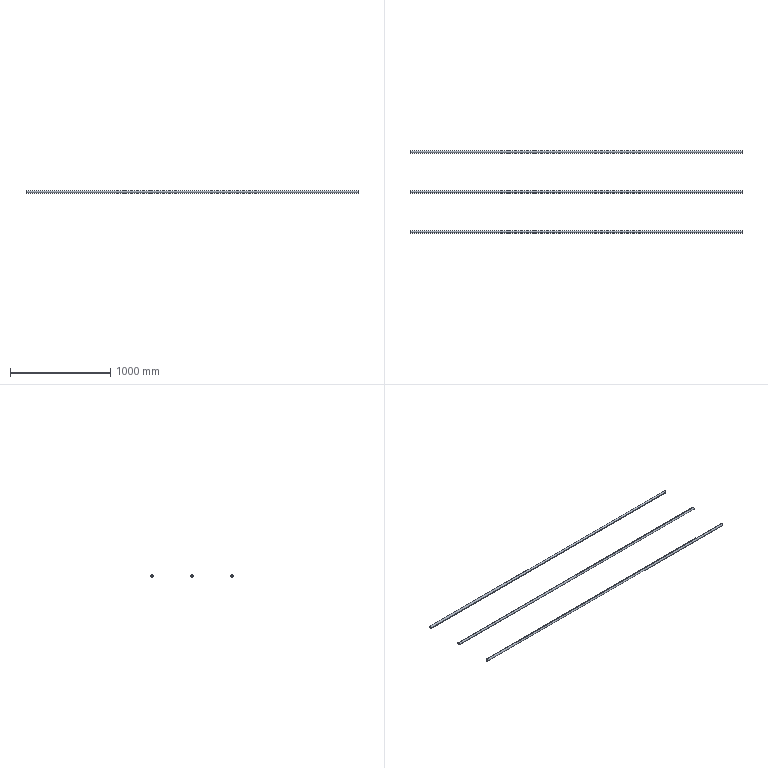Part | STEP file | E3-电柜护栏5栏杆_Default<As Machined> | 3 solids | 18 faces | box 3320 x 825 x 25 mm | volume 1102982 mm3 | cylinder 12 | plane 6 | commonest cylinder face diameters 22 x6 25 x6
STEP:
#1=CARTESIAN_POINT('',(0.,0.,0.));
#2=DIRECTION('',(0.,0.,1.));
#3=DIRECTION('',(1.,0.,0.));
#4=AXIS2_PLACEMENT_3D('',#1,#2,#3);
#5=CARTESIAN_POINT('',(-3320.,0.,12.5));
#6=VERTEX_POINT('',#5);
#7=CARTESIAN_POINT('',(-3320.,0.,-12.5));
#8=VERTEX_POINT('',#7);
#9=CARTESIAN_POINT('',(-3320.,0.,0.));
#10=DIRECTION('',(1.,0.,0.));
#11=DIRECTION('',(0.,-1.,0.));
#12=AXIS2_PLACEMENT_3D('',#9,#10,#11);
#13=CIRCLE('',#12,12.5);
#14=CARTESIAN_POINT('',(-3320.,0.,0.));
#15=DIRECTION('',(1.,0.,0.));
#16=DIRECTION('',(0.,0.,1.));
#17=AXIS2_PLACEMENT_3D('',#14,#15,#16);
#18=CYLINDRICAL_SURFACE('',#17,12.5);
#19=CARTESIAN_POINT('',(-4.712,0.));
#20=DIRECTION('',(1.,0.));
#21=VECTOR('',#20,1.);
#22=LINE('',#19,#21);
#23=(GEOMETRIC_REPRESENTATION_CONTEXT(2)PARAMETRIC_REPRESENTATION_CONTEXT()REPRESENTATION_CONTEXT('',''));
#24=DEFINITIONAL_REPRESENTATION('',(#22),#23);
#25=PCURVE('',#18,#24);
#26=CARTESIAN_POINT('',(-3320.,0.,0.));
#27=DIRECTION('',(-1.,0.,0.));
#28=DIRECTION('',(0.,-1.,0.));
#29=AXIS2_PLACEMENT_3D('',#26,#27,#28);
#30=PLANE('',#29);
#31=CARTESIAN_POINT('',(12.5,0.));
#32=CARTESIAN_POINT('',(12.5,-21.651));
#33=CARTESIAN_POINT('',(-6.25,-10.825));
#34=CARTESIAN_POINT('',(-25.,0.));
#35=CARTESIAN_POINT('',(-6.25,10.825));
#36=CARTESIAN_POINT('',(12.5,21.651));
#37=CARTESIAN_POINT('',(12.5,0.));
#38=(BOUNDED_CURVE()B_SPLINE_CURVE(2,(#31,#32,#33,#34,#35,#36,#37),.UNSPECIFIED.,.T.,.F.)B_SPLINE_CURVE_WITH_KNOTS((1,2,2,2,2,1),(-2.094,0.,2.094,4.189,6.283,8.378),.UNSPECIFIED.)CURVE()GEOMETRIC_REPRESENTATION_ITEM()RATIONAL_B_SPLINE_CURVE((1.,0.5,1.,0.5,1.,0.5,1.))REPRESENTATION_ITEM(''));
#39=(GEOMETRIC_REPRESENTATION_CONTEXT(2)PARAMETRIC_REPRESENTATION_CONTEXT()REPRESENTATION_CONTEXT('',''));
#40=DEFINITIONAL_REPRESENTATION('',(#38),#39);
#41=PCURVE('',#30,#40);
#42=SURFACE_CURVE('',#13,(#25,#41),.PCURVE_S1.);
#43=EDGE_CURVE('',#6,#8,#42,.T.);
#44=ORIENTED_EDGE('',*,*,#43,.T.);
#45=CARTESIAN_POINT('',(0.,0.,-12.5));
#46=VERTEX_POINT('',#45);
#47=CARTESIAN_POINT('',(-3320.,0.,-12.5));
#48=DIRECTION('',(1.,0.,0.));
#49=VECTOR('',#48,1.);
#50=LINE('',#47,#49);
#51=CARTESIAN_POINT('',(3.142,0.));
#52=DIRECTION('',(0.,1.));
#53=VECTOR('',#52,1.);
#54=LINE('',#51,#53);
#55=(GEOMETRIC_REPRESENTATION_CONTEXT(2)PARAMETRIC_REPRESENTATION_CONTEXT()REPRESENTATION_CONTEXT('',''));
#56=DEFINITIONAL_REPRESENTATION('',(#54),#55);
#57=PCURVE('',#18,#56);
#58=CARTESIAN_POINT('',(-3320.,0.,0.));
#59=DIRECTION('',(1.,0.,0.));
#60=DIRECTION('',(0.,0.,1.));
#61=AXIS2_PLACEMENT_3D('',#58,#59,#60);
#62=CYLINDRICAL_SURFACE('',#61,12.5);
#63=CARTESIAN_POINT('',(3.142,0.));
#64=DIRECTION('',(0.,1.));
#65=VECTOR('',#64,1.);
#66=LINE('',#63,#65);
#67=(GEOMETRIC_REPRESENTATION_CONTEXT(2)PARAMETRIC_REPRESENTATION_CONTEXT()REPRESENTATION_CONTEXT('',''));
#68=DEFINITIONAL_REPRESENTATION('',(#66),#67);
#69=PCURVE('',#62,#68);
#70=SURFACE_CURVE('',#50,(#57,#69),.PCURVE_S1.);
#71=EDGE_CURVE('',#8,#46,#70,.T.);
#72=ORIENTED_EDGE('',*,*,#71,.T.);
#73=CARTESIAN_POINT('',(0.,0.,12.5));
#74=VERTEX_POINT('',#73);
#75=CARTESIAN_POINT('',(0.,0.,0.));
#76=DIRECTION('',(1.,0.,0.));
#77=DIRECTION('',(0.,-1.,0.));
#78=AXIS2_PLACEMENT_3D('',#75,#76,#77);
#79=CIRCLE('',#78,12.5);
#80=CARTESIAN_POINT('',(-4.712,3320.));
#81=DIRECTION('',(1.,0.));
#82=VECTOR('',#81,1.);
#83=LINE('',#80,#82);
#84=(GEOMETRIC_REPRESENTATION_CONTEXT(2)PARAMETRIC_REPRESENTATION_CONTEXT()REPRESENTATION_CONTEXT('',''));
#85=DEFINITIONAL_REPRESENTATION('',(#83),#84);
#86=PCURVE('',#18,#85);
#87=CARTESIAN_POINT('',(0.,0.,0.));
#88=DIRECTION('',(-1.,0.,0.));
#89=DIRECTION('',(0.,-1.,0.));
#90=AXIS2_PLACEMENT_3D('',#87,#88,#89);
#91=PLANE('',#90);
#92=CARTESIAN_POINT('',(12.5,0.));
#93=CARTESIAN_POINT('',(12.5,-21.651));
#94=CARTESIAN_POINT('',(-6.25,-10.825));
#95=CARTESIAN_POINT('',(-25.,0.));
#96=CARTESIAN_POINT('',(-6.25,10.825));
#97=CARTESIAN_POINT('',(12.5,21.651));
#98=CARTESIAN_POINT('',(12.5,0.));
#99=(BOUNDED_CURVE()B_SPLINE_CURVE(2,(#92,#93,#94,#95,#96,#97,#98),.UNSPECIFIED.,.T.,.F.)B_SPLINE_CURVE_WITH_KNOTS((1,2,2,2,2,1),(-2.094,0.,2.094,4.189,6.283,8.378),.UNSPECIFIED.)CURVE()GEOMETRIC_REPRESENTATION_ITEM()RATIONAL_B_SPLINE_CURVE((1.,0.5,1.,0.5,1.,0.5,1.))REPRESENTATION_ITEM(''));
#100=(GEOMETRIC_REPRESENTATION_CONTEXT(2)PARAMETRIC_REPRESENTATION_CONTEXT()REPRESENTATION_CONTEXT('',''));
#101=DEFINITIONAL_REPRESENTATION('',(#99),#100);
#102=PCURVE('',#91,#101);
#103=SURFACE_CURVE('',#79,(#86,#102),.PCURVE_S1.);
#104=EDGE_CURVE('',#74,#46,#103,.T.);
#105=ORIENTED_EDGE('',*,*,#104,.F.);
#106=CARTESIAN_POINT('',(-3320.,0.,12.5));
#107=DIRECTION('',(1.,0.,0.));
#108=VECTOR('',#107,1.);
#109=LINE('',#106,#108);
#110=CARTESIAN_POINT('',(0.,0.));
#111=DIRECTION('',(0.,1.));
#112=VECTOR('',#111,1.);
#113=LINE('',#110,#112);
#114=(GEOMETRIC_REPRESENTATION_CONTEXT(2)PARAMETRIC_REPRESENTATION_CONTEXT()REPRESENTATION_CONTEXT('',''));
#115=DEFINITIONAL_REPRESENTATION('',(#113),#114);
#116=PCURVE('',#18,#115);
#117=CARTESIAN_POINT('',(6.283,0.));
#118=DIRECTION('',(0.,1.));
#119=VECTOR('',#118,1.);
#120=LINE('',#117,#119);
#121=(GEOMETRIC_REPRESENTATION_CONTEXT(2)PARAMETRIC_REPRESENTATION_CONTEXT()REPRESENTATION_CONTEXT('',''));
#122=DEFINITIONAL_REPRESENTATION('',(#120),#121);
#123=PCURVE('',#62,#122);
#124=SURFACE_CURVE('',#109,(#116,#123),.PCURVE_S1.);
#125=EDGE_CURVE('',#6,#74,#124,.T.);
#126=ORIENTED_EDGE('',*,*,#125,.F.);
#127=EDGE_LOOP('',(#44,#72,#105,#126));
#128=FACE_BOUND('',#127,.T.);
#129=ADVANCED_FACE('',(#128),#18,.T.);
#130=CARTESIAN_POINT('',(-3320.,0.,11.));
#131=VERTEX_POINT('',#130);
#132=CARTESIAN_POINT('',(0.,0.,11.));
#133=VERTEX_POINT('',#132);
#134=CARTESIAN_POINT('',(-3320.,0.,11.));
#135=DIRECTION('',(1.,0.,0.));
#136=VECTOR('',#135,1.);
#137=LINE('',#134,#136);
#138=CARTESIAN_POINT('',(-3320.,0.,0.));
#139=DIRECTION('',(1.,0.,0.));
#140=DIRECTION('',(0.,0.,1.));
#141=AXIS2_PLACEMENT_3D('',#138,#139,#140);
#142=CYLINDRICAL_SURFACE('',#141,11.);
#143=CARTESIAN_POINT('',(6.283,0.));
#144=DIRECTION('',(0.,1.));
#145=VECTOR('',#144,1.);
#146=LINE('',#143,#145);
#147=(GEOMETRIC_REPRESENTATION_CONTEXT(2)PARAMETRIC_REPRESENTATION_CONTEXT()REPRESENTATION_CONTEXT('',''));
#148=DEFINITIONAL_REPRESENTATION('',(#146),#147);
#149=PCURVE('',#142,#148);
#150=CARTESIAN_POINT('',(-3320.,0.,0.));
#151=DIRECTION('',(1.,0.,0.));
#152=DIRECTION('',(0.,0.,1.));
#153=AXIS2_PLACEMENT_3D('',#150,#151,#152);
#154=CYLINDRICAL_SURFACE('',#153,11.);
#155=CARTESIAN_POINT('',(0.,0.));
#156=DIRECTION('',(0.,1.));
#157=VECTOR('',#156,1.);
#158=LINE('',#155,#157);
#159=(GEOMETRIC_REPRESENTATION_CONTEXT(2)PARAMETRIC_REPRESENTATION_CONTEXT()REPRESENTATION_CONTEXT('',''));
#160=DEFINITIONAL_REPRESENTATION('',(#158),#159);
#161=PCURVE('',#154,#160);
#162=SURFACE_CURVE('',#137,(#149,#161),.PCURVE_S1.);
#163=EDGE_CURVE('',#131,#133,#162,.T.);
#164=ORIENTED_EDGE('',*,*,#163,.T.);
#165=CARTESIAN_POINT('',(0.,0.,-11.));
#166=VERTEX_POINT('',#165);
#167=CARTESIAN_POINT('',(0.,0.,0.));
#168=DIRECTION('',(1.,0.,0.));
#169=DIRECTION('',(0.,-1.,0.));
#170=AXIS2_PLACEMENT_3D('',#167,#168,#169);
#171=CIRCLE('',#170,11.);
#172=CARTESIAN_POINT('',(1.571,3320.));
#173=DIRECTION('',(1.,0.));
#174=VECTOR('',#173,1.);
#175=LINE('',#172,#174);
#176=(GEOMETRIC_REPRESENTATION_CONTEXT(2)PARAMETRIC_REPRESENTATION_CONTEXT()REPRESENTATION_CONTEXT('',''));
#177=DEFINITIONAL_REPRESENTATION('',(#175),#176);
#178=PCURVE('',#142,#177);
#179=CARTESIAN_POINT('',(11.,0.));
#180=CARTESIAN_POINT('',(11.,-19.053));
#181=CARTESIAN_POINT('',(-5.5,-9.526));
#182=CARTESIAN_POINT('',(-22.,0.));
#183=CARTESIAN_POINT('',(-5.5,9.526));
#184=CARTESIAN_POINT('',(11.,19.053));
#185=CARTESIAN_POINT('',(11.,0.));
#186=(BOUNDED_CURVE()B_SPLINE_CURVE(2,(#179,#180,#181,#182,#183,#184,#185),.UNSPECIFIED.,.T.,.F.)B_SPLINE_CURVE_WITH_KNOTS((1,2,2,2,2,1),(-2.094,0.,2.094,4.189,6.283,8.378),.UNSPECIFIED.)CURVE()GEOMETRIC_REPRESENTATION_ITEM()RATIONAL_B_SPLINE_CURVE((1.,0.5,1.,0.5,1.,0.5,1.))REPRESENTATION_ITEM(''));
#187=(GEOMETRIC_REPRESENTATION_CONTEXT(2)PARAMETRIC_REPRESENTATION_CONTEXT()REPRESENTATION_CONTEXT('',''));
#188=DEFINITIONAL_REPRESENTATION('',(#186),#187);
#189=PCURVE('',#91,#188);
#190=SURFACE_CURVE('',#171,(#178,#189),.PCURVE_S1.);
#191=EDGE_CURVE('',#166,#133,#190,.T.);
#192=ORIENTED_EDGE('',*,*,#191,.F.);
#193=CARTESIAN_POINT('',(-3320.,0.,-11.));
#194=VERTEX_POINT('',#193);
#195=CARTESIAN_POINT('',(-3320.,0.,-11.));
#196=DIRECTION('',(1.,0.,0.));
#197=VECTOR('',#196,1.);
#198=LINE('',#195,#197);
#199=CARTESIAN_POINT('',(3.142,0.));
#200=DIRECTION('',(0.,1.));
#201=VECTOR('',#200,1.);
#202=LINE('',#199,#201);
#203=(GEOMETRIC_REPRESENTATION_CONTEXT(2)PARAMETRIC_REPRESENTATION_CONTEXT()REPRESENTATION_CONTEXT('',''));
#204=DEFINITIONAL_REPRESENTATION('',(#202),#203);
#205=PCURVE('',#142,#204);
#206=CARTESIAN_POINT('',(3.142,0.));
#207=DIRECTION('',(0.,1.));
#208=VECTOR('',#207,1.);
#209=LINE('',#206,#208);
#210=(GEOMETRIC_REPRESENTATION_CONTEXT(2)PARAMETRIC_REPRESENTATION_CONTEXT()REPRESENTATION_CONTEXT('',''));
#211=DEFINITIONAL_REPRESENTATION('',(#209),#210);
#212=PCURVE('',#154,#211);
#213=SURFACE_CURVE('',#198,(#205,#212),.PCURVE_S1.);
#214=EDGE_CURVE('',#194,#166,#213,.T.);
#215=ORIENTED_EDGE('',*,*,#214,.F.);
#216=CARTESIAN_POINT('',(-3320.,0.,0.));
#217=DIRECTION('',(1.,0.,0.));
#218=DIRECTION('',(0.,-1.,0.));
#219=AXIS2_PLACEMENT_3D('',#216,#217,#218);
#220=CIRCLE('',#219,11.);
#221=CARTESIAN_POINT('',(1.571,0.));
#222=DIRECTION('',(1.,0.));
#223=VECTOR('',#222,1.);
#224=LINE('',#221,#223);
#225=(GEOMETRIC_REPRESENTATION_CONTEXT(2)PARAMETRIC_REPRESENTATION_CONTEXT()REPRESENTATION_CONTEXT('',''));
#226=DEFINITIONAL_REPRESENTATION('',(#224),#225);
#227=PCURVE('',#142,#226);
#228=CARTESIAN_POINT('',(11.,0.));
#229=CARTESIAN_POINT('',(11.,-19.053));
#230=CARTESIAN_POINT('',(-5.5,-9.526));
#231=CARTESIAN_POINT('',(-22.,0.));
#232=CARTESIAN_POINT('',(-5.5,9.526));
#233=CARTESIAN_POINT('',(11.,19.053));
#234=CARTESIAN_POINT('',(11.,0.));
#235=(BOUNDED_CURVE()B_SPLINE_CURVE(2,(#228,#229,#230,#231,#232,#233,#234),.UNSPECIFIED.,.T.,.F.)B_SPLINE_CURVE_WITH_KNOTS((1,2,2,2,2,1),(-2.094,0.,2.094,4.189,6.283,8.378),.UNSPECIFIED.)CURVE()GEOMETRIC_REPRESENTATION_ITEM()RATIONAL_B_SPLINE_CURVE((1.,0.5,1.,0.5,1.,0.5,1.))REPRESENTATION_ITEM(''));
#236=(GEOMETRIC_REPRESENTATION_CONTEXT(2)PARAMETRIC_REPRESENTATION_CONTEXT()REPRESENTATION_CONTEXT('',''));
#237=DEFINITIONAL_REPRESENTATION('',(#235),#236);
#238=PCURVE('',#30,#237);
#239=SURFACE_CURVE('',#220,(#227,#238),.PCURVE_S1.);
#240=EDGE_CURVE('',#194,#131,#239,.T.);
#241=ORIENTED_EDGE('',*,*,#240,.T.);
#242=EDGE_LOOP('',(#164,#192,#215,#241));
#243=FACE_BOUND('',#242,.F.);
#244=ADVANCED_FACE('',(#243),#142,.F.);
#245=CARTESIAN_POINT('',(0.,0.,0.));
#246=DIRECTION('',(1.,0.,0.));
#247=DIRECTION('',(0.,-1.,0.));
#248=AXIS2_PLACEMENT_3D('',#245,#246,#247);
#249=CIRCLE('',#248,11.);
#250=CARTESIAN_POINT('',(-4.712,3320.));
#251=DIRECTION('',(1.,0.));
#252=VECTOR('',#251,1.);
#253=LINE('',#250,#252);
#254=(GEOMETRIC_REPRESENTATION_CONTEXT(2)PARAMETRIC_REPRESENTATION_CONTEXT()REPRESENTATION_CONTEXT('',''));
#255=DEFINITIONAL_REPRESENTATION('',(#253),#254);
#256=PCURVE('',#154,#255);
#257=CARTESIAN_POINT('',(11.,0.));
#258=CARTESIAN_POINT('',(11.,-19.053));
#259=CARTESIAN_POINT('',(-5.5,-9.526));
#260=CARTESIAN_POINT('',(-22.,0.));
#261=CARTESIAN_POINT('',(-5.5,9.526));
#262=CARTESIAN_POINT('',(11.,19.053));
#263=CARTESIAN_POINT('',(11.,0.));
#264=(BOUNDED_CURVE()B_SPLINE_CURVE(2,(#257,#258,#259,#260,#261,#262,#263),.UNSPECIFIED.,.T.,.F.)B_SPLINE_CURVE_WITH_KNOTS((1,2,2,2,2,1),(-2.094,0.,2.094,4.189,6.283,8.378),.UNSPECIFIED.)CURVE()GEOMETRIC_REPRESENTATION_ITEM()RATIONAL_B_SPLINE_CURVE((1.,0.5,1.,0.5,1.,0.5,1.))REPRESENTATION_ITEM(''));
#265=(GEOMETRIC_REPRESENTATION_CONTEXT(2)PARAMETRIC_REPRESENTATION_CONTEXT()REPRESENTATION_CONTEXT('',''));
#266=DEFINITIONAL_REPRESENTATION('',(#264),#265);
#267=PCURVE('',#91,#266);
#268=SURFACE_CURVE('',#249,(#256,#267),.PCURVE_S1.);
#269=EDGE_CURVE('',#133,#166,#268,.T.);
#270=ORIENTED_EDGE('',*,*,#269,.F.);
#271=ORIENTED_EDGE('',*,*,#163,.F.);
#272=CARTESIAN_POINT('',(-3320.,0.,0.));
#273=DIRECTION('',(1.,0.,0.));
#274=DIRECTION('',(0.,-1.,0.));
#275=AXIS2_PLACEMENT_3D('',#272,#273,#274);
#276=CIRCLE('',#275,11.);
#277=CARTESIAN_POINT('',(-4.712,0.));
#278=DIRECTION('',(1.,0.));
#279=VECTOR('',#278,1.);
#280=LINE('',#277,#279);
#281=(GEOMETRIC_REPRESENTATION_CONTEXT(2)PARAMETRIC_REPRESENTATION_CONTEXT()REPRESENTATION_CONTEXT('',''));
#282=DEFINITIONAL_REPRESENTATION('',(#280),#281);
#283=PCURVE('',#154,#282);
#284=CARTESIAN_POINT('',(11.,0.));
#285=CARTESIAN_POINT('',(11.,-19.053));
#286=CARTESIAN_POINT('',(-5.5,-9.526));
#287=CARTESIAN_POINT('',(-22.,0.));
#288=CARTESIAN_POINT('',(-5.5,9.526));
#289=CARTESIAN_POINT('',(11.,19.053));
#290=CARTESIAN_POINT('',(11.,0.));
#291=(BOUNDED_CURVE()B_SPLINE_CURVE(2,(#284,#285,#286,#287,#288,#289,#290),.UNSPECIFIED.,.T.,.F.)B_SPLINE_CURVE_WITH_KNOTS((1,2,2,2,2,1),(-2.094,0.,2.094,4.189,6.283,8.378),.UNSPECIFIED.)CURVE()GEOMETRIC_REPRESENTATION_ITEM()RATIONAL_B_SPLINE_CURVE((1.,0.5,1.,0.5,1.,0.5,1.))REPRESENTATION_ITEM(''));
#292=(GEOMETRIC_REPRESENTATION_CONTEXT(2)PARAMETRIC_REPRESENTATION_CONTEXT()REPRESENTATION_CONTEXT('',''));
#293=DEFINITIONAL_REPRESENTATION('',(#291),#292);
#294=PCURVE('',#30,#293);
#295=SURFACE_CURVE('',#276,(#283,#294),.PCURVE_S1.);
#296=EDGE_CURVE('',#131,#194,#295,.T.);
#297=ORIENTED_EDGE('',*,*,#296,.T.);
#298=ORIENTED_EDGE('',*,*,#214,.T.);
#299=EDGE_LOOP('',(#270,#271,#297,#298));
#300=FACE_BOUND('',#299,.F.);
#301=ADVANCED_FACE('',(#300),#154,.F.);
#302=ORIENTED_EDGE('',*,*,#71,.F.);
#303=CARTESIAN_POINT('',(-3320.,0.,0.));
#304=DIRECTION('',(1.,0.,0.));
#305=DIRECTION('',(0.,-1.,0.));
#306=AXIS2_PLACEMENT_3D('',#303,#304,#305);
#307=CIRCLE('',#306,12.5);
#308=CARTESIAN_POINT('',(1.571,0.));
#309=DIRECTION('',(1.,0.));
#310=VECTOR('',#309,1.);
#311=LINE('',#308,#310);
#312=(GEOMETRIC_REPRESENTATION_CONTEXT(2)PARAMETRIC_REPRESENTATION_CONTEXT()REPRESENTATION_CONTEXT('',''));
#313=DEFINITIONAL_REPRESENTATION('',(#311),#312);
#314=PCURVE('',#62,#313);
#315=CARTESIAN_POINT('',(12.5,0.));
#316=CARTESIAN_POINT('',(12.5,-21.651));
#317=CARTESIAN_POINT('',(-6.25,-10.825));
#318=CARTESIAN_POINT('',(-25.,0.));
#319=CARTESIAN_POINT('',(-6.25,10.825));
#320=CARTESIAN_POINT('',(12.5,21.651));
#321=CARTESIAN_POINT('',(12.5,0.));
#322=(BOUNDED_CURVE()B_SPLINE_CURVE(2,(#315,#316,#317,#318,#319,#320,#321),.UNSPECIFIED.,.T.,.F.)B_SPLINE_CURVE_WITH_KNOTS((1,2,2,2,2,1),(-2.094,0.,2.094,4.189,6.283,8.378),.UNSPECIFIED.)CURVE()GEOMETRIC_REPRESENTATION_ITEM()RATIONAL_B_SPLINE_CURVE((1.,0.5,1.,0.5,1.,0.5,1.))REPRESENTATION_ITEM(''));
#323=(GEOMETRIC_REPRESENTATION_CONTEXT(2)PARAMETRIC_REPRESENTATION_CONTEXT()REPRESENTATION_CONTEXT('',''));
#324=DEFINITIONAL_REPRESENTATION('',(#322),#323);
#325=PCURVE('',#30,#324);
#326=SURFACE_CURVE('',#307,(#314,#325),.PCURVE_S1.);
#327=EDGE_CURVE('',#8,#6,#326,.T.);
#328=ORIENTED_EDGE('',*,*,#327,.T.);
#329=ORIENTED_EDGE('',*,*,#125,.T.);
#330=CARTESIAN_POINT('',(0.,0.,0.));
#331=DIRECTION('',(1.,0.,0.));
#332=DIRECTION('',(0.,-1.,0.));
#333=AXIS2_PLACEMENT_3D('',#330,#331,#332);
#334=CIRCLE('',#333,12.5);
#335=CARTESIAN_POINT('',(1.571,3320.));
#336=DIRECTION('',(1.,0.));
#337=VECTOR('',#336,1.);
#338=LINE('',#335,#337);
#339=(GEOMETRIC_REPRESENTATION_CONTEXT(2)PARAMETRIC_REPRESENTATION_CONTEXT()REPRESENTATION_CONTEXT('',''));
#340=DEFINITIONAL_REPRESENTATION('',(#338),#339);
#341=PCURVE('',#62,#340);
#342=CARTESIAN_POINT('',(12.5,0.));
#343=CARTESIAN_POINT('',(12.5,-21.651));
#344=CARTESIAN_POINT('',(-6.25,-10.825));
#345=CARTESIAN_POINT('',(-25.,0.));
#346=CARTESIAN_POINT('',(-6.25,10.825));
#347=CARTESIAN_POINT('',(12.5,21.651));
#348=CARTESIAN_POINT('',(12.5,0.));
#349=(BOUNDED_CURVE()B_SPLINE_CURVE(2,(#342,#343,#344,#345,#346,#347,#348),.UNSPECIFIED.,.T.,.F.)B_SPLINE_CURVE_WITH_KNOTS((1,2,2,2,2,1),(-2.094,0.,2.094,4.189,6.283,8.378),.UNSPECIFIED.)CURVE()GEOMETRIC_REPRESENTATION_ITEM()RATIONAL_B_SPLINE_CURVE((1.,0.5,1.,0.5,1.,0.5,1.))REPRESENTATION_ITEM(''));
#350=(GEOMETRIC_REPRESENTATION_CONTEXT(2)PARAMETRIC_REPRESENTATION_CONTEXT()REPRESENTATION_CONTEXT('',''));
#351=DEFINITIONAL_REPRESENTATION('',(#349),#350);
#352=PCURVE('',#91,#351);
#353=SURFACE_CURVE('',#334,(#341,#352),.PCURVE_S1.);
#354=EDGE_CURVE('',#46,#74,#353,.T.);
#355=ORIENTED_EDGE('',*,*,#354,.F.);
#356=EDGE_LOOP('',(#302,#328,#329,#355));
#357=FACE_BOUND('',#356,.T.);
#358=ADVANCED_FACE('',(#357),#62,.T.);
#359=ORIENTED_EDGE('',*,*,#296,.T.);
#360=ORIENTED_EDGE('',*,*,#240,.T.);
#361=EDGE_LOOP('',(#359,#360));
#362=FACE_BOUND('',#361,.T.);
#363=ORIENTED_EDGE('',*,*,#43,.F.);
#364=ORIENTED_EDGE('',*,*,#327,.F.);
#365=EDGE_LOOP('',(#363,#364));
#366=FACE_BOUND('',#365,.T.);
#367=ADVANCED_FACE('',(#362,#366),#30,.T.);
#368=ORIENTED_EDGE('',*,*,#269,.F.);
#369=ORIENTED_EDGE('',*,*,#191,.F.);
#370=EDGE_LOOP('',(#368,#369));
#371=FACE_BOUND('',#370,.T.);
#372=ORIENTED_EDGE('',*,*,#104,.T.);
#373=ORIENTED_EDGE('',*,*,#354,.T.);
#374=EDGE_LOOP('',(#372,#373));
#375=FACE_BOUND('',#374,.T.);
#376=ADVANCED_FACE('',(#371,#375),#91,.F.);
#377=CLOSED_SHELL('',(#129,#244,#301,#358,#367,#376));
#378=MANIFOLD_SOLID_BREP('',#377);
#379=CARTESIAN_POINT('',(-3320.,812.5,0.));
#380=VERTEX_POINT('',#379);
#381=CARTESIAN_POINT('',(-3320.,787.5,0.));
#382=VERTEX_POINT('',#381);
#383=CARTESIAN_POINT('',(-3320.,800.,0.));
#384=DIRECTION('',(1.,0.,0.));
#385=DIRECTION('',(0.,-1.,0.));
#386=AXIS2_PLACEMENT_3D('',#383,#384,#385);
#387=CIRCLE('',#386,12.5);
#388=CARTESIAN_POINT('',(-3320.,800.,0.));
#389=DIRECTION('',(1.,0.,0.));
#390=DIRECTION('',(0.,1.,0.));
#391=AXIS2_PLACEMENT_3D('',#388,#389,#390);
#392=CYLINDRICAL_SURFACE('',#391,12.5);
#393=CARTESIAN_POINT('',(-3.142,0.));
#394=DIRECTION('',(1.,0.));
#395=VECTOR('',#394,1.);
#396=LINE('',#393,#395);
#397=(GEOMETRIC_REPRESENTATION_CONTEXT(2)PARAMETRIC_REPRESENTATION_CONTEXT()REPRESENTATION_CONTEXT('',''));
#398=DEFINITIONAL_REPRESENTATION('',(#396),#397);
#399=PCURVE('',#392,#398);
#400=CARTESIAN_POINT('',(-3320.,800.,0.));
#401=DIRECTION('',(-1.,0.,0.));
#402=DIRECTION('',(0.,-1.,0.));
#403=AXIS2_PLACEMENT_3D('',#400,#401,#402);
#404=PLANE('',#403);
#405=CARTESIAN_POINT('',(12.5,0.));
#406=CARTESIAN_POINT('',(12.5,-21.651));
#407=CARTESIAN_POINT('',(-6.25,-10.825));
#408=CARTESIAN_POINT('',(-25.,0.));
#409=CARTESIAN_POINT('',(-6.25,10.825));
#410=CARTESIAN_POINT('',(12.5,21.651));
#411=CARTESIAN_POINT('',(12.5,0.));
#412=(BOUNDED_CURVE()B_SPLINE_CURVE(2,(#405,#406,#407,#408,#409,#410,#411),.UNSPECIFIED.,.T.,.F.)B_SPLINE_CURVE_WITH_KNOTS((1,2,2,2,2,1),(-2.094,0.,2.094,4.189,6.283,8.378),.UNSPECIFIED.)CURVE()GEOMETRIC_REPRESENTATION_ITEM()RATIONAL_B_SPLINE_CURVE((1.,0.5,1.,0.5,1.,0.5,1.))REPRESENTATION_ITEM(''));
#413=(GEOMETRIC_REPRESENTATION_CONTEXT(2)PARAMETRIC_REPRESENTATION_CONTEXT()REPRESENTATION_CONTEXT('',''));
#414=DEFINITIONAL_REPRESENTATION('',(#412),#413);
#415=PCURVE('',#404,#414);
#416=SURFACE_CURVE('',#387,(#399,#415),.PCURVE_S1.);
#417=EDGE_CURVE('',#380,#382,#416,.T.);
#418=ORIENTED_EDGE('',*,*,#417,.T.);
#419=CARTESIAN_POINT('',(0.,787.5,0.));
#420=VERTEX_POINT('',#419);
#421=CARTESIAN_POINT('',(-3320.,787.5,0.));
#422=DIRECTION('',(1.,0.,0.));
#423=VECTOR('',#422,1.);
#424=LINE('',#421,#423);
#425=CARTESIAN_POINT('',(3.142,0.));
#426=DIRECTION('',(0.,1.));
#427=VECTOR('',#426,1.);
#428=LINE('',#425,#427);
#429=(GEOMETRIC_REPRESENTATION_CONTEXT(2)PARAMETRIC_REPRESENTATION_CONTEXT()REPRESENTATION_CONTEXT('',''));
#430=DEFINITIONAL_REPRESENTATION('',(#428),#429);
#431=PCURVE('',#392,#430);
#432=CARTESIAN_POINT('',(-3320.,800.,0.));
#433=DIRECTION('',(1.,0.,0.));
#434=DIRECTION('',(0.,1.,0.));
#435=AXIS2_PLACEMENT_3D('',#432,#433,#434);
#436=CYLINDRICAL_SURFACE('',#435,12.5);
#437=CARTESIAN_POINT('',(3.142,0.));
#438=DIRECTION('',(0.,1.));
#439=VECTOR('',#438,1.);
#440=LINE('',#437,#439);
#441=(GEOMETRIC_REPRESENTATION_CONTEXT(2)PARAMETRIC_REPRESENTATION_CONTEXT()REPRESENTATION_CONTEXT('',''));
#442=DEFINITIONAL_REPRESENTATION('',(#440),#441);
#443=PCURVE('',#436,#442);
#444=SURFACE_CURVE('',#424,(#431,#443),.PCURVE_S1.);
#445=EDGE_CURVE('',#382,#420,#444,.T.);
#446=ORIENTED_EDGE('',*,*,#445,.T.);
#447=CARTESIAN_POINT('',(0.,812.5,0.));
#448=VERTEX_POINT('',#447);
#449=CARTESIAN_POINT('',(0.,800.,0.));
#450=DIRECTION('',(1.,0.,0.));
#451=DIRECTION('',(0.,-1.,0.));
#452=AXIS2_PLACEMENT_3D('',#449,#450,#451);
#453=CIRCLE('',#452,12.5);
#454=CARTESIAN_POINT('',(-3.142,3320.));
#455=DIRECTION('',(1.,0.));
#456=VECTOR('',#455,1.);
#457=LINE('',#454,#456);
#458=(GEOMETRIC_REPRESENTATION_CONTEXT(2)PARAMETRIC_REPRESENTATION_CONTEXT()REPRESENTATION_CONTEXT('',''));
#459=DEFINITIONAL_REPRESENTATION('',(#457),#458);
#460=PCURVE('',#392,#459);
#461=CARTESIAN_POINT('',(0.,800.,0.));
#462=DIRECTION('',(-1.,0.,0.));
#463=DIRECTION('',(0.,-1.,0.));
#464=AXIS2_PLACEMENT_3D('',#461,#462,#463);
#465=PLANE('',#464);
#466=CARTESIAN_POINT('',(12.5,0.));
#467=CARTESIAN_POINT('',(12.5,-21.651));
#468=CARTESIAN_POINT('',(-6.25,-10.825));
#469=CARTESIAN_POINT('',(-25.,0.));
#470=CARTESIAN_POINT('',(-6.25,10.825));
#471=CARTESIAN_POINT('',(12.5,21.651));
#472=CARTESIAN_POINT('',(12.5,0.));
#473=(BOUNDED_CURVE()B_SPLINE_CURVE(2,(#466,#467,#468,#469,#470,#471,#472),.UNSPECIFIED.,.T.,.F.)B_SPLINE_CURVE_WITH_KNOTS((1,2,2,2,2,1),(-2.094,0.,2.094,4.189,6.283,8.378),.UNSPECIFIED.)CURVE()GEOMETRIC_REPRESENTATION_ITEM()RATIONAL_B_SPLINE_CURVE((1.,0.5,1.,0.5,1.,0.5,1.))REPRESENTATION_ITEM(''));
#474=(GEOMETRIC_REPRESENTATION_CONTEXT(2)PARAMETRIC_REPRESENTATION_CONTEXT()REPRESENTATION_CONTEXT('',''));
#475=DEFINITIONAL_REPRESENTATION('',(#473),#474);
#476=PCURVE('',#465,#475);
#477=SURFACE_CURVE('',#453,(#460,#476),.PCURVE_S1.);
#478=EDGE_CURVE('',#448,#420,#477,.T.);
#479=ORIENTED_EDGE('',*,*,#478,.F.);
#480=CARTESIAN_POINT('',(-3320.,812.5,0.));
#481=DIRECTION('',(1.,0.,0.));
#482=VECTOR('',#481,1.);
#483=LINE('',#480,#482);
#484=CARTESIAN_POINT('',(0.,0.));
#485=DIRECTION('',(0.,1.));
#486=VECTOR('',#485,1.);
#487=LINE('',#484,#486);
#488=(GEOMETRIC_REPRESENTATION_CONTEXT(2)PARAMETRIC_REPRESENTATION_CONTEXT()REPRESENTATION_CONTEXT('',''));
#489=DEFINITIONAL_REPRESENTATION('',(#487),#488);
#490=PCURVE('',#392,#489);
#491=CARTESIAN_POINT('',(6.283,0.));
#492=DIRECTION('',(0.,1.));
#493=VECTOR('',#492,1.);
#494=LINE('',#491,#493);
#495=(GEOMETRIC_REPRESENTATION_CONTEXT(2)PARAMETRIC_REPRESENTATION_CONTEXT()REPRESENTATION_CONTEXT('',''));
#496=DEFINITIONAL_REPRESENTATION('',(#494),#495);
#497=PCURVE('',#436,#496);
#498=SURFACE_CURVE('',#483,(#490,#497),.PCURVE_S1.);
#499=EDGE_CURVE('',#380,#448,#498,.T.);
#500=ORIENTED_EDGE('',*,*,#499,.F.);
#501=EDGE_LOOP('',(#418,#446,#479,#500));
#502=FACE_BOUND('',#501,.T.);
#503=ADVANCED_FACE('',(#502),#392,.T.);
#504=CARTESIAN_POINT('',(-3320.,811.,0.));
#505=VERTEX_POINT('',#504);
#506=CARTESIAN_POINT('',(0.,811.,0.));
#507=VERTEX_POINT('',#506);
#508=CARTESIAN_POINT('',(-3320.,811.,0.));
#509=DIRECTION('',(1.,0.,0.));
#510=VECTOR('',#509,1.);
#511=LINE('',#508,#510);
#512=CARTESIAN_POINT('',(-3320.,800.,0.));
#513=DIRECTION('',(1.,0.,0.));
#514=DIRECTION('',(0.,1.,0.));
#515=AXIS2_PLACEMENT_3D('',#512,#513,#514);
#516=CYLINDRICAL_SURFACE('',#515,11.);
#517=CARTESIAN_POINT('',(6.283,0.));
#518=DIRECTION('',(0.,1.));
#519=VECTOR('',#518,1.);
#520=LINE('',#517,#519);
#521=(GEOMETRIC_REPRESENTATION_CONTEXT(2)PARAMETRIC_REPRESENTATION_CONTEXT()REPRESENTATION_CONTEXT('',''));
#522=DEFINITIONAL_REPRESENTATION('',(#520),#521);
#523=PCURVE('',#516,#522);
#524=CARTESIAN_POINT('',(-3320.,800.,0.));
#525=DIRECTION('',(1.,0.,0.));
#526=DIRECTION('',(0.,1.,0.));
#527=AXIS2_PLACEMENT_3D('',#524,#525,#526);
#528=CYLINDRICAL_SURFACE('',#527,11.);
#529=CARTESIAN_POINT('',(0.,0.));
#530=DIRECTION('',(0.,1.));
#531=VECTOR('',#530,1.);
#532=LINE('',#529,#531);
#533=(GEOMETRIC_REPRESENTATION_CONTEXT(2)PARAMETRIC_REPRESENTATION_CONTEXT()REPRESENTATION_CONTEXT('',''));
#534=DEFINITIONAL_REPRESENTATION('',(#532),#533);
#535=PCURVE('',#528,#534);
#536=SURFACE_CURVE('',#511,(#523,#535),.PCURVE_S1.);
#537=EDGE_CURVE('',#505,#507,#536,.T.);
#538=ORIENTED_EDGE('',*,*,#537,.T.);
#539=CARTESIAN_POINT('',(0.,789.,0.));
#540=VERTEX_POINT('',#539);
#541=CARTESIAN_POINT('',(0.,800.,0.));
#542=DIRECTION('',(1.,0.,0.));
#543=DIRECTION('',(0.,-1.,0.));
#544=AXIS2_PLACEMENT_3D('',#541,#542,#543);
#545=CIRCLE('',#544,11.);
#546=CARTESIAN_POINT('',(3.142,3320.));
#547=DIRECTION('',(1.,0.));
#548=VECTOR('',#547,1.);
#549=LINE('',#546,#548);
#550=(GEOMETRIC_REPRESENTATION_CONTEXT(2)PARAMETRIC_REPRESENTATION_CONTEXT()REPRESENTATION_CONTEXT('',''));
#551=DEFINITIONAL_REPRESENTATION('',(#549),#550);
#552=PCURVE('',#516,#551);
#553=CARTESIAN_POINT('',(11.,0.));
#554=CARTESIAN_POINT('',(11.,-19.053));
#555=CARTESIAN_POINT('',(-5.5,-9.526));
#556=CARTESIAN_POINT('',(-22.,0.));
#557=CARTESIAN_POINT('',(-5.5,9.526));
#558=CARTESIAN_POINT('',(11.,19.053));
#559=CARTESIAN_POINT('',(11.,0.));
#560=(BOUNDED_CURVE()B_SPLINE_CURVE(2,(#553,#554,#555,#556,#557,#558,#559),.UNSPECIFIED.,.T.,.F.)B_SPLINE_CURVE_WITH_KNOTS((1,2,2,2,2,1),(-2.094,0.,2.094,4.189,6.283,8.378),.UNSPECIFIED.)CURVE()GEOMETRIC_REPRESENTATION_ITEM()RATIONAL_B_SPLINE_CURVE((1.,0.5,1.,0.5,1.,0.5,1.))REPRESENTATION_ITEM(''));
#561=(GEOMETRIC_REPRESENTATION_CONTEXT(2)PARAMETRIC_REPRESENTATION_CONTEXT()REPRESENTATION_CONTEXT('',''));
#562=DEFINITIONAL_REPRESENTATION('',(#560),#561);
#563=PCURVE('',#465,#562);
#564=SURFACE_CURVE('',#545,(#552,#563),.PCURVE_S1.);
#565=EDGE_CURVE('',#540,#507,#564,.T.);
#566=ORIENTED_EDGE('',*,*,#565,.F.);
#567=CARTESIAN_POINT('',(-3320.,789.,0.));
#568=VERTEX_POINT('',#567);
#569=CARTESIAN_POINT('',(-3320.,789.,0.));
#570=DIRECTION('',(1.,0.,0.));
#571=VECTOR('',#570,1.);
#572=LINE('',#569,#571);
#573=CARTESIAN_POINT('',(3.142,0.));
#574=DIRECTION('',(0.,1.));
#575=VECTOR('',#574,1.);
#576=LINE('',#573,#575);
#577=(GEOMETRIC_REPRESENTATION_CONTEXT(2)PARAMETRIC_REPRESENTATION_CONTEXT()REPRESENTATION_CONTEXT('',''));
#578=DEFINITIONAL_REPRESENTATION('',(#576),#577);
#579=PCURVE('',#516,#578);
#580=CARTESIAN_POINT('',(3.142,0.));
#581=DIRECTION('',(0.,1.));
#582=VECTOR('',#581,1.);
#583=LINE('',#580,#582);
#584=(GEOMETRIC_REPRESENTATION_CONTEXT(2)PARAMETRIC_REPRESENTATION_CONTEXT()REPRESENTATION_CONTEXT('',''));
#585=DEFINITIONAL_REPRESENTATION('',(#583),#584);
#586=PCURVE('',#528,#585);
#587=SURFACE_CURVE('',#572,(#579,#586),.PCURVE_S1.);
#588=EDGE_CURVE('',#568,#540,#587,.T.);
#589=ORIENTED_EDGE('',*,*,#588,.F.);
#590=CARTESIAN_POINT('',(-3320.,800.,0.));
#591=DIRECTION('',(1.,0.,0.));
#592=DIRECTION('',(0.,-1.,0.));
#593=AXIS2_PLACEMENT_3D('',#590,#591,#592);
#594=CIRCLE('',#593,11.);
#595=CARTESIAN_POINT('',(3.142,0.));
#596=DIRECTION('',(1.,0.));
#597=VECTOR('',#596,1.);
#598=LINE('',#595,#597);
#599=(GEOMETRIC_REPRESENTATION_CONTEXT(2)PARAMETRIC_REPRESENTATION_CONTEXT()REPRESENTATION_CONTEXT('',''));
#600=DEFINITIONAL_REPRESENTATION('',(#598),#599);
#601=PCURVE('',#516,#600);
#602=CARTESIAN_POINT('',(11.,0.));
#603=CARTESIAN_POINT('',(11.,-19.053));
#604=CARTESIAN_POINT('',(-5.5,-9.526));
#605=CARTESIAN_POINT('',(-22.,0.));
#606=CARTESIAN_POINT('',(-5.5,9.526));
#607=CARTESIAN_POINT('',(11.,19.053));
#608=CARTESIAN_POINT('',(11.,0.));
#609=(BOUNDED_CURVE()B_SPLINE_CURVE(2,(#602,#603,#604,#605,#606,#607,#608),.UNSPECIFIED.,.T.,.F.)B_SPLINE_CURVE_WITH_KNOTS((1,2,2,2,2,1),(-2.094,0.,2.094,4.189,6.283,8.378),.UNSPECIFIED.)CURVE()GEOMETRIC_REPRESENTATION_ITEM()RATIONAL_B_SPLINE_CURVE((1.,0.5,1.,0.5,1.,0.5,1.))REPRESENTATION_ITEM(''));
#610=(GEOMETRIC_REPRESENTATION_CONTEXT(2)PARAMETRIC_REPRESENTATION_CONTEXT()REPRESENTATION_CONTEXT('',''));
#611=DEFINITIONAL_REPRESENTATION('',(#609),#610);
#612=PCURVE('',#404,#611);
#613=SURFACE_CURVE('',#594,(#601,#612),.PCURVE_S1.);
#614=EDGE_CURVE('',#568,#505,#613,.T.);
#615=ORIENTED_EDGE('',*,*,#614,.T.);
#616=EDGE_LOOP('',(#538,#566,#589,#615));
#617=FACE_BOUND('',#616,.F.);
#618=ADVANCED_FACE('',(#617),#516,.F.);
#619=CARTESIAN_POINT('',(0.,800.,0.));
#620=DIRECTION('',(1.,0.,0.));
#621=DIRECTION('',(0.,-1.,0.));
#622=AXIS2_PLACEMENT_3D('',#619,#620,#621);
#623=CIRCLE('',#622,11.);
#624=CARTESIAN_POINT('',(-3.142,3320.));
#625=DIRECTION('',(1.,0.));
#626=VECTOR('',#625,1.);
#627=LINE('',#624,#626);
#628=(GEOMETRIC_REPRESENTATION_CONTEXT(2)PARAMETRIC_REPRESENTATION_CONTEXT()REPRESENTATION_CONTEXT('',''));
#629=DEFINITIONAL_REPRESENTATION('',(#627),#628);
#630=PCURVE('',#528,#629);
#631=CARTESIAN_POINT('',(11.,0.));
#632=CARTESIAN_POINT('',(11.,-19.053));
#633=CARTESIAN_POINT('',(-5.5,-9.526));
#634=CARTESIAN_POINT('',(-22.,0.));
#635=CARTESIAN_POINT('',(-5.5,9.526));
#636=CARTESIAN_POINT('',(11.,19.053));
#637=CARTESIAN_POINT('',(11.,0.));
#638=(BOUNDED_CURVE()B_SPLINE_CURVE(2,(#631,#632,#633,#634,#635,#636,#637),.UNSPECIFIED.,.T.,.F.)B_SPLINE_CURVE_WITH_KNOTS((1,2,2,2,2,1),(-2.094,0.,2.094,4.189,6.283,8.378),.UNSPECIFIED.)CURVE()GEOMETRIC_REPRESENTATION_ITEM()RATIONAL_B_SPLINE_CURVE((1.,0.5,1.,0.5,1.,0.5,1.))REPRESENTATION_ITEM(''));
#639=(GEOMETRIC_REPRESENTATION_CONTEXT(2)PARAMETRIC_REPRESENTATION_CONTEXT()REPRESENTATION_CONTEXT('',''));
#640=DEFINITIONAL_REPRESENTATION('',(#638),#639);
#641=PCURVE('',#465,#640);
#642=SURFACE_CURVE('',#623,(#630,#641),.PCURVE_S1.);
#643=EDGE_CURVE('',#507,#540,#642,.T.);
#644=ORIENTED_EDGE('',*,*,#643,.F.);
#645=ORIENTED_EDGE('',*,*,#537,.F.);
#646=CARTESIAN_POINT('',(-3320.,800.,0.));
#647=DIRECTION('',(1.,0.,0.));
#648=DIRECTION('',(0.,-1.,0.));
#649=AXIS2_PLACEMENT_3D('',#646,#647,#648);
#650=CIRCLE('',#649,11.);
#651=CARTESIAN_POINT('',(-3.142,0.));
#652=DIRECTION('',(1.,0.));
#653=VECTOR('',#652,1.);
#654=LINE('',#651,#653);
#655=(GEOMETRIC_REPRESENTATION_CONTEXT(2)PARAMETRIC_REPRESENTATION_CONTEXT()REPRESENTATION_CONTEXT('',''));
#656=DEFINITIONAL_REPRESENTATION('',(#654),#655);
#657=PCURVE('',#528,#656);
#658=CARTESIAN_POINT('',(11.,0.));
#659=CARTESIAN_POINT('',(11.,-19.053));
#660=CARTESIAN_POINT('',(-5.5,-9.526));
#661=CARTESIAN_POINT('',(-22.,0.));
#662=CARTESIAN_POINT('',(-5.5,9.526));
#663=CARTESIAN_POINT('',(11.,19.053));
#664=CARTESIAN_POINT('',(11.,0.));
#665=(BOUNDED_CURVE()B_SPLINE_CURVE(2,(#658,#659,#660,#661,#662,#663,#664),.UNSPECIFIED.,.T.,.F.)B_SPLINE_CURVE_WITH_KNOTS((1,2,2,2,2,1),(-2.094,0.,2.094,4.189,6.283,8.378),.UNSPECIFIED.)CURVE()GEOMETRIC_REPRESENTATION_ITEM()RATIONAL_B_SPLINE_CURVE((1.,0.5,1.,0.5,1.,0.5,1.))REPRESENTATION_ITEM(''));
#666=(GEOMETRIC_REPRESENTATION_CONTEXT(2)PARAMETRIC_REPRESENTATION_CONTEXT()REPRESENTATION_CONTEXT('',''));
#667=DEFINITIONAL_REPRESENTATION('',(#665),#666);
#668=PCURVE('',#404,#667);
#669=SURFACE_CURVE('',#650,(#657,#668),.PCURVE_S1.);
#670=EDGE_CURVE('',#505,#568,#669,.T.);
#671=ORIENTED_EDGE('',*,*,#670,.T.);
#672=ORIENTED_EDGE('',*,*,#588,.T.);
#673=EDGE_LOOP('',(#644,#645,#671,#672));
#674=FACE_BOUND('',#673,.F.);
#675=ADVANCED_FACE('',(#674),#528,.F.);
#676=ORIENTED_EDGE('',*,*,#445,.F.);
#677=CARTESIAN_POINT('',(-3320.,800.,0.));
#678=DIRECTION('',(1.,0.,0.));
#679=DIRECTION('',(0.,-1.,0.));
#680=AXIS2_PLACEMENT_3D('',#677,#678,#679);
#681=CIRCLE('',#680,12.5);
#682=CARTESIAN_POINT('',(3.142,0.));
#683=DIRECTION('',(1.,0.));
#684=VECTOR('',#683,1.);
#685=LINE('',#682,#684);
#686=(GEOMETRIC_REPRESENTATION_CONTEXT(2)PARAMETRIC_REPRESENTATION_CONTEXT()REPRESENTATION_CONTEXT('',''));
#687=DEFINITIONAL_REPRESENTATION('',(#685),#686);
#688=PCURVE('',#436,#687);
#689=CARTESIAN_POINT('',(12.5,0.));
#690=CARTESIAN_POINT('',(12.5,-21.651));
#691=CARTESIAN_POINT('',(-6.25,-10.825));
#692=CARTESIAN_POINT('',(-25.,0.));
#693=CARTESIAN_POINT('',(-6.25,10.825));
#694=CARTESIAN_POINT('',(12.5,21.651));
#695=CARTESIAN_POINT('',(12.5,0.));
#696=(BOUNDED_CURVE()B_SPLINE_CURVE(2,(#689,#690,#691,#692,#693,#694,#695),.UNSPECIFIED.,.T.,.F.)B_SPLINE_CURVE_WITH_KNOTS((1,2,2,2,2,1),(-2.094,0.,2.094,4.189,6.283,8.378),.UNSPECIFIED.)CURVE()GEOMETRIC_REPRESENTATION_ITEM()RATIONAL_B_SPLINE_CURVE((1.,0.5,1.,0.5,1.,0.5,1.))REPRESENTATION_ITEM(''));
#697=(GEOMETRIC_REPRESENTATION_CONTEXT(2)PARAMETRIC_REPRESENTATION_CONTEXT()REPRESENTATION_CONTEXT('',''));
#698=DEFINITIONAL_REPRESENTATION('',(#696),#697);
#699=PCURVE('',#404,#698);
#700=SURFACE_CURVE('',#681,(#688,#699),.PCURVE_S1.);
#701=EDGE_CURVE('',#382,#380,#700,.T.);
#702=ORIENTED_EDGE('',*,*,#701,.T.);
#703=ORIENTED_EDGE('',*,*,#499,.T.);
#704=CARTESIAN_POINT('',(0.,800.,0.));
#705=DIRECTION('',(1.,0.,0.));
#706=DIRECTION('',(0.,-1.,0.));
#707=AXIS2_PLACEMENT_3D('',#704,#705,#706);
#708=CIRCLE('',#707,12.5);
#709=CARTESIAN_POINT('',(3.142,3320.));
#710=DIRECTION('',(1.,0.));
#711=VECTOR('',#710,1.);
#712=LINE('',#709,#711);
#713=(GEOMETRIC_REPRESENTATION_CONTEXT(2)PARAMETRIC_REPRESENTATION_CONTEXT()REPRESENTATION_CONTEXT('',''));
#714=DEFINITIONAL_REPRESENTATION('',(#712),#713);
#715=PCURVE('',#436,#714);
#716=CARTESIAN_POINT('',(12.5,0.));
#717=CARTESIAN_POINT('',(12.5,-21.651));
#718=CARTESIAN_POINT('',(-6.25,-10.825));
#719=CARTESIAN_POINT('',(-25.,0.));
#720=CARTESIAN_POINT('',(-6.25,10.825));
#721=CARTESIAN_POINT('',(12.5,21.651));
#722=CARTESIAN_POINT('',(12.5,0.));
#723=(BOUNDED_CURVE()B_SPLINE_CURVE(2,(#716,#717,#718,#719,#720,#721,#722),.UNSPECIFIED.,.T.,.F.)B_SPLINE_CURVE_WITH_KNOTS((1,2,2,2,2,1),(-2.094,0.,2.094,4.189,6.283,8.378),.UNSPECIFIED.)CURVE()GEOMETRIC_REPRESENTATION_ITEM()RATIONAL_B_SPLINE_CURVE((1.,0.5,1.,0.5,1.,0.5,1.))REPRESENTATION_ITEM(''));
#724=(GEOMETRIC_REPRESENTATION_CONTEXT(2)PARAMETRIC_REPRESENTATION_CONTEXT()REPRESENTATION_CONTEXT('',''));
#725=DEFINITIONAL_REPRESENTATION('',(#723),#724);
#726=PCURVE('',#465,#725);
#727=SURFACE_CURVE('',#708,(#715,#726),.PCURVE_S1.);
#728=EDGE_CURVE('',#420,#448,#727,.T.);
#729=ORIENTED_EDGE('',*,*,#728,.F.);
#730=EDGE_LOOP('',(#676,#702,#703,#729));
#731=FACE_BOUND('',#730,.T.);
#732=ADVANCED_FACE('',(#731),#436,.T.);
#733=ORIENTED_EDGE('',*,*,#670,.T.);
#734=ORIENTED_EDGE('',*,*,#614,.T.);
#735=EDGE_LOOP('',(#733,#734));
#736=FACE_BOUND('',#735,.T.);
#737=ORIENTED_EDGE('',*,*,#417,.F.);
#738=ORIENTED_EDGE('',*,*,#701,.F.);
#739=EDGE_LOOP('',(#737,#738));
#740=FACE_BOUND('',#739,.T.);
#741=ADVANCED_FACE('',(#736,#740),#404,.T.);
#742=ORIENTED_EDGE('',*,*,#643,.F.);
#743=ORIENTED_EDGE('',*,*,#565,.F.);
#744=EDGE_LOOP('',(#742,#743));
#745=FACE_BOUND('',#744,.T.);
#746=ORIENTED_EDGE('',*,*,#478,.T.);
#747=ORIENTED_EDGE('',*,*,#728,.T.);
#748=EDGE_LOOP('',(#746,#747));
#749=FACE_BOUND('',#748,.T.);
#750=ADVANCED_FACE('',(#745,#749),#465,.F.);
#751=CLOSED_SHELL('',(#503,#618,#675,#732,#741,#750));
#752=MANIFOLD_SOLID_BREP('',#751);
#753=CARTESIAN_POINT('',(0.,400.,-12.5));
#754=VERTEX_POINT('',#753);
#755=CARTESIAN_POINT('',(0.,400.,12.5));
#756=VERTEX_POINT('',#755);
#757=CARTESIAN_POINT('',(0.,400.,0.));
#758=DIRECTION('',(-1.,0.,0.));
#759=DIRECTION('',(0.,1.,0.));
#760=AXIS2_PLACEMENT_3D('',#757,#758,#759);
#761=CIRCLE('',#760,12.5);
#762=CARTESIAN_POINT('',(0.,400.,0.));
#763=DIRECTION('',(-1.,0.,0.));
#764=DIRECTION('',(0.,0.,-1.));
#765=AXIS2_PLACEMENT_3D('',#762,#763,#764);
#766=CYLINDRICAL_SURFACE('',#765,12.5);
#767=CARTESIAN_POINT('',(-1.571,0.));
#768=DIRECTION('',(1.,0.));
#769=VECTOR('',#768,1.);
#770=LINE('',#767,#769);
#771=(GEOMETRIC_REPRESENTATION_CONTEXT(2)PARAMETRIC_REPRESENTATION_CONTEXT()REPRESENTATION_CONTEXT('',''));
#772=DEFINITIONAL_REPRESENTATION('',(#770),#771);
#773=PCURVE('',#766,#772);
#774=CARTESIAN_POINT('',(0.,400.,0.));
#775=DIRECTION('',(1.,0.,0.));
#776=DIRECTION('',(0.,1.,0.));
#777=AXIS2_PLACEMENT_3D('',#774,#775,#776);
#778=PLANE('',#777);
#779=CARTESIAN_POINT('',(12.5,0.));
#780=CARTESIAN_POINT('',(12.5,-21.651));
#781=CARTESIAN_POINT('',(-6.25,-10.825));
#782=CARTESIAN_POINT('',(-25.,0.));
#783=CARTESIAN_POINT('',(-6.25,10.825));
#784=CARTESIAN_POINT('',(12.5,21.651));
#785=CARTESIAN_POINT('',(12.5,0.));
#786=(BOUNDED_CURVE()B_SPLINE_CURVE(2,(#779,#780,#781,#782,#783,#784,#785),.UNSPECIFIED.,.T.,.F.)B_SPLINE_CURVE_WITH_KNOTS((1,2,2,2,2,1),(-2.094,0.,2.094,4.189,6.283,8.378),.UNSPECIFIED.)CURVE()GEOMETRIC_REPRESENTATION_ITEM()RATIONAL_B_SPLINE_CURVE((1.,0.5,1.,0.5,1.,0.5,1.))REPRESENTATION_ITEM(''));
#787=(GEOMETRIC_REPRESENTATION_CONTEXT(2)PARAMETRIC_REPRESENTATION_CONTEXT()REPRESENTATION_CONTEXT('',''));
#788=DEFINITIONAL_REPRESENTATION('',(#786),#787);
#789=PCURVE('',#778,#788);
#790=SURFACE_CURVE('',#761,(#773,#789),.PCURVE_S1.);
#791=EDGE_CURVE('',#754,#756,#790,.T.);
#792=ORIENTED_EDGE('',*,*,#791,.T.);
#793=CARTESIAN_POINT('',(-3320.,400.,12.5));
#794=VERTEX_POINT('',#793);
#795=CARTESIAN_POINT('',(0.,400.,12.5));
#796=DIRECTION('',(-1.,0.,0.));
#797=VECTOR('',#796,1.);
#798=LINE('',#795,#797);
#799=CARTESIAN_POINT('',(3.142,0.));
#800=DIRECTION('',(0.,1.));
#801=VECTOR('',#800,1.);
#802=LINE('',#799,#801);
#803=(GEOMETRIC_REPRESENTATION_CONTEXT(2)PARAMETRIC_REPRESENTATION_CONTEXT()REPRESENTATION_CONTEXT('',''));
#804=DEFINITIONAL_REPRESENTATION('',(#802),#803);
#805=PCURVE('',#766,#804);
#806=CARTESIAN_POINT('',(0.,400.,0.));
#807=DIRECTION('',(-1.,0.,0.));
#808=DIRECTION('',(0.,0.,-1.));
#809=AXIS2_PLACEMENT_3D('',#806,#807,#808);
#810=CYLINDRICAL_SURFACE('',#809,12.5);
#811=CARTESIAN_POINT('',(3.142,0.));
#812=DIRECTION('',(0.,1.));
#813=VECTOR('',#812,1.);
#814=LINE('',#811,#813);
#815=(GEOMETRIC_REPRESENTATION_CONTEXT(2)PARAMETRIC_REPRESENTATION_CONTEXT()REPRESENTATION_CONTEXT('',''));
#816=DEFINITIONAL_REPRESENTATION('',(#814),#815);
#817=PCURVE('',#810,#816);
#818=SURFACE_CURVE('',#798,(#805,#817),.PCURVE_S1.);
#819=EDGE_CURVE('',#756,#794,#818,.T.);
#820=ORIENTED_EDGE('',*,*,#819,.T.);
#821=CARTESIAN_POINT('',(-3320.,400.,-12.5));
#822=VERTEX_POINT('',#821);
#823=CARTESIAN_POINT('',(-3320.,400.,0.));
#824=DIRECTION('',(-1.,0.,0.));
#825=DIRECTION('',(0.,1.,0.));
#826=AXIS2_PLACEMENT_3D('',#823,#824,#825);
#827=CIRCLE('',#826,12.5);
#828=CARTESIAN_POINT('',(-1.571,3320.));
#829=DIRECTION('',(1.,0.));
#830=VECTOR('',#829,1.);
#831=LINE('',#828,#830);
#832=(GEOMETRIC_REPRESENTATION_CONTEXT(2)PARAMETRIC_REPRESENTATION_CONTEXT()REPRESENTATION_CONTEXT('',''));
#833=DEFINITIONAL_REPRESENTATION('',(#831),#832);
#834=PCURVE('',#766,#833);
#835=CARTESIAN_POINT('',(-3320.,400.,0.));
#836=DIRECTION('',(1.,0.,0.));
#837=DIRECTION('',(0.,1.,0.));
#838=AXIS2_PLACEMENT_3D('',#835,#836,#837);
#839=PLANE('',#838);
#840=CARTESIAN_POINT('',(12.5,0.));
#841=CARTESIAN_POINT('',(12.5,-21.651));
#842=CARTESIAN_POINT('',(-6.25,-10.825));
#843=CARTESIAN_POINT('',(-25.,0.));
#844=CARTESIAN_POINT('',(-6.25,10.825));
#845=CARTESIAN_POINT('',(12.5,21.651));
#846=CARTESIAN_POINT('',(12.5,0.));
#847=(BOUNDED_CURVE()B_SPLINE_CURVE(2,(#840,#841,#842,#843,#844,#845,#846),.UNSPECIFIED.,.T.,.F.)B_SPLINE_CURVE_WITH_KNOTS((1,2,2,2,2,1),(-2.094,0.,2.094,4.189,6.283,8.378),.UNSPECIFIED.)CURVE()GEOMETRIC_REPRESENTATION_ITEM()RATIONAL_B_SPLINE_CURVE((1.,0.5,1.,0.5,1.,0.5,1.))REPRESENTATION_ITEM(''));
#848=(GEOMETRIC_REPRESENTATION_CONTEXT(2)PARAMETRIC_REPRESENTATION_CONTEXT()REPRESENTATION_CONTEXT('',''));
#849=DEFINITIONAL_REPRESENTATION('',(#847),#848);
#850=PCURVE('',#839,#849);
#851=SURFACE_CURVE('',#827,(#834,#850),.PCURVE_S1.);
#852=EDGE_CURVE('',#822,#794,#851,.T.);
#853=ORIENTED_EDGE('',*,*,#852,.F.);
#854=CARTESIAN_POINT('',(0.,400.,-12.5));
#855=DIRECTION('',(-1.,0.,0.));
#856=VECTOR('',#855,1.);
#857=LINE('',#854,#856);
#858=CARTESIAN_POINT('',(0.,0.));
#859=DIRECTION('',(0.,1.));
#860=VECTOR('',#859,1.);
#861=LINE('',#858,#860);
#862=(GEOMETRIC_REPRESENTATION_CONTEXT(2)PARAMETRIC_REPRESENTATION_CONTEXT()REPRESENTATION_CONTEXT('',''));
#863=DEFINITIONAL_REPRESENTATION('',(#861),#862);
#864=PCURVE('',#766,#863);
#865=CARTESIAN_POINT('',(6.283,0.));
#866=DIRECTION('',(0.,1.));
#867=VECTOR('',#866,1.);
#868=LINE('',#865,#867);
#869=(GEOMETRIC_REPRESENTATION_CONTEXT(2)PARAMETRIC_REPRESENTATION_CONTEXT()REPRESENTATION_CONTEXT('',''));
#870=DEFINITIONAL_REPRESENTATION('',(#868),#869);
#871=PCURVE('',#810,#870);
#872=SURFACE_CURVE('',#857,(#864,#871),.PCURVE_S1.);
#873=EDGE_CURVE('',#754,#822,#872,.T.);
#874=ORIENTED_EDGE('',*,*,#873,.F.);
#875=EDGE_LOOP('',(#792,#820,#853,#874));
#876=FACE_BOUND('',#875,.T.);
#877=ADVANCED_FACE('',(#876),#766,.T.);
#878=CARTESIAN_POINT('',(0.,400.,-11.));
#879=VERTEX_POINT('',#878);
#880=CARTESIAN_POINT('',(-3320.,400.,-11.));
#881=VERTEX_POINT('',#880);
#882=CARTESIAN_POINT('',(0.,400.,-11.));
#883=DIRECTION('',(-1.,0.,0.));
#884=VECTOR('',#883,1.);
#885=LINE('',#882,#884);
#886=CARTESIAN_POINT('',(0.,400.,0.));
#887=DIRECTION('',(-1.,0.,0.));
#888=DIRECTION('',(0.,0.,-1.));
#889=AXIS2_PLACEMENT_3D('',#886,#887,#888);
#890=CYLINDRICAL_SURFACE('',#889,11.);
#891=CARTESIAN_POINT('',(6.283,0.));
#892=DIRECTION('',(0.,1.));
#893=VECTOR('',#892,1.);
#894=LINE('',#891,#893);
#895=(GEOMETRIC_REPRESENTATION_CONTEXT(2)PARAMETRIC_REPRESENTATION_CONTEXT()REPRESENTATION_CONTEXT('',''));
#896=DEFINITIONAL_REPRESENTATION('',(#894),#895);
#897=PCURVE('',#890,#896);
#898=CARTESIAN_POINT('',(0.,400.,0.));
#899=DIRECTION('',(-1.,0.,0.));
#900=DIRECTION('',(0.,0.,-1.));
#901=AXIS2_PLACEMENT_3D('',#898,#899,#900);
#902=CYLINDRICAL_SURFACE('',#901,11.);
#903=CARTESIAN_POINT('',(0.,0.));
#904=DIRECTION('',(0.,1.));
#905=VECTOR('',#904,1.);
#906=LINE('',#903,#905);
#907=(GEOMETRIC_REPRESENTATION_CONTEXT(2)PARAMETRIC_REPRESENTATION_CONTEXT()REPRESENTATION_CONTEXT('',''));
#908=DEFINITIONAL_REPRESENTATION('',(#906),#907);
#909=PCURVE('',#902,#908);
#910=SURFACE_CURVE('',#885,(#897,#909),.PCURVE_S1.);
#911=EDGE_CURVE('',#879,#881,#910,.T.);
#912=ORIENTED_EDGE('',*,*,#911,.T.);
#913=CARTESIAN_POINT('',(-3320.,400.,11.));
#914=VERTEX_POINT('',#913);
#915=CARTESIAN_POINT('',(-3320.,400.,0.));
#916=DIRECTION('',(-1.,0.,0.));
#917=DIRECTION('',(0.,1.,0.));
#918=AXIS2_PLACEMENT_3D('',#915,#916,#917);
#919=CIRCLE('',#918,11.);
#920=CARTESIAN_POINT('',(-1.571,3320.));
#921=DIRECTION('',(1.,0.));
#922=VECTOR('',#921,1.);
#923=LINE('',#920,#922);
#924=(GEOMETRIC_REPRESENTATION_CONTEXT(2)PARAMETRIC_REPRESENTATION_CONTEXT()REPRESENTATION_CONTEXT('',''));
#925=DEFINITIONAL_REPRESENTATION('',(#923),#924);
#926=PCURVE('',#890,#925);
#927=CARTESIAN_POINT('',(11.,0.));
#928=CARTESIAN_POINT('',(11.,-19.053));
#929=CARTESIAN_POINT('',(-5.5,-9.526));
#930=CARTESIAN_POINT('',(-22.,0.));
#931=CARTESIAN_POINT('',(-5.5,9.526));
#932=CARTESIAN_POINT('',(11.,19.053));
#933=CARTESIAN_POINT('',(11.,0.));
#934=(BOUNDED_CURVE()B_SPLINE_CURVE(2,(#927,#928,#929,#930,#931,#932,#933),.UNSPECIFIED.,.T.,.F.)B_SPLINE_CURVE_WITH_KNOTS((1,2,2,2,2,1),(-2.094,0.,2.094,4.189,6.283,8.378),.UNSPECIFIED.)CURVE()GEOMETRIC_REPRESENTATION_ITEM()RATIONAL_B_SPLINE_CURVE((1.,0.5,1.,0.5,1.,0.5,1.))REPRESENTATION_ITEM(''));
#935=(GEOMETRIC_REPRESENTATION_CONTEXT(2)PARAMETRIC_REPRESENTATION_CONTEXT()REPRESENTATION_CONTEXT('',''));
#936=DEFINITIONAL_REPRESENTATION('',(#934),#935);
#937=PCURVE('',#839,#936);
#938=SURFACE_CURVE('',#919,(#926,#937),.PCURVE_S1.);
#939=EDGE_CURVE('',#914,#881,#938,.T.);
#940=ORIENTED_EDGE('',*,*,#939,.F.);
#941=CARTESIAN_POINT('',(0.,400.,11.));
#942=VERTEX_POINT('',#941);
#943=CARTESIAN_POINT('',(0.,400.,11.));
#944=DIRECTION('',(-1.,0.,0.));
#945=VECTOR('',#944,1.);
#946=LINE('',#943,#945);
#947=CARTESIAN_POINT('',(3.142,0.));
#948=DIRECTION('',(0.,1.));
#949=VECTOR('',#948,1.);
#950=LINE('',#947,#949);
#951=(GEOMETRIC_REPRESENTATION_CONTEXT(2)PARAMETRIC_REPRESENTATION_CONTEXT()REPRESENTATION_CONTEXT('',''));
#952=DEFINITIONAL_REPRESENTATION('',(#950),#951);
#953=PCURVE('',#890,#952);
#954=CARTESIAN_POINT('',(3.142,0.));
#955=DIRECTION('',(0.,1.));
#956=VECTOR('',#955,1.);
#957=LINE('',#954,#956);
#958=(GEOMETRIC_REPRESENTATION_CONTEXT(2)PARAMETRIC_REPRESENTATION_CONTEXT()REPRESENTATION_CONTEXT('',''));
#959=DEFINITIONAL_REPRESENTATION('',(#957),#958);
#960=PCURVE('',#902,#959);
#961=SURFACE_CURVE('',#946,(#953,#960),.PCURVE_S1.);
#962=EDGE_CURVE('',#942,#914,#961,.T.);
#963=ORIENTED_EDGE('',*,*,#962,.F.);
#964=CARTESIAN_POINT('',(0.,400.,0.));
#965=DIRECTION('',(-1.,0.,0.));
#966=DIRECTION('',(0.,1.,0.));
#967=AXIS2_PLACEMENT_3D('',#964,#965,#966);
#968=CIRCLE('',#967,11.);
#969=CARTESIAN_POINT('',(-1.571,0.));
#970=DIRECTION('',(1.,0.));
#971=VECTOR('',#970,1.);
#972=LINE('',#969,#971);
#973=(GEOMETRIC_REPRESENTATION_CONTEXT(2)PARAMETRIC_REPRESENTATION_CONTEXT()REPRESENTATION_CONTEXT('',''));
#974=DEFINITIONAL_REPRESENTATION('',(#972),#973);
#975=PCURVE('',#890,#974);
#976=CARTESIAN_POINT('',(11.,0.));
#977=CARTESIAN_POINT('',(11.,-19.053));
#978=CARTESIAN_POINT('',(-5.5,-9.526));
#979=CARTESIAN_POINT('',(-22.,0.));
#980=CARTESIAN_POINT('',(-5.5,9.526));
#981=CARTESIAN_POINT('',(11.,19.053));
#982=CARTESIAN_POINT('',(11.,0.));
#983=(BOUNDED_CURVE()B_SPLINE_CURVE(2,(#976,#977,#978,#979,#980,#981,#982),.UNSPECIFIED.,.T.,.F.)B_SPLINE_CURVE_WITH_KNOTS((1,2,2,2,2,1),(-2.094,0.,2.094,4.189,6.283,8.378),.UNSPECIFIED.)CURVE()GEOMETRIC_REPRESENTATION_ITEM()RATIONAL_B_SPLINE_CURVE((1.,0.5,1.,0.5,1.,0.5,1.))REPRESENTATION_ITEM(''));
#984=(GEOMETRIC_REPRESENTATION_CONTEXT(2)PARAMETRIC_REPRESENTATION_CONTEXT()REPRESENTATION_CONTEXT('',''));
#985=DEFINITIONAL_REPRESENTATION('',(#983),#984);
#986=PCURVE('',#778,#985);
#987=SURFACE_CURVE('',#968,(#975,#986),.PCURVE_S1.);
#988=EDGE_CURVE('',#942,#879,#987,.T.);
#989=ORIENTED_EDGE('',*,*,#988,.T.);
#990=EDGE_LOOP('',(#912,#940,#963,#989));
#991=FACE_BOUND('',#990,.F.);
#992=ADVANCED_FACE('',(#991),#890,.F.);
#993=CARTESIAN_POINT('',(-3320.,400.,0.));
#994=DIRECTION('',(-1.,0.,0.));
#995=DIRECTION('',(0.,1.,0.));
#996=AXIS2_PLACEMENT_3D('',#993,#994,#995);
#997=CIRCLE('',#996,11.);
#998=CARTESIAN_POINT('',(-1.571,3320.));
#999=DIRECTION('',(1.,0.));
#1000=VECTOR('',#999,1.);
#1001=LINE('',#998,#1000);
#1002=(GEOMETRIC_REPRESENTATION_CONTEXT(2)PARAMETRIC_REPRESENTATION_CONTEXT()REPRESENTATION_CONTEXT('',''));
#1003=DEFINITIONAL_REPRESENTATION('',(#1001),#1002);
#1004=PCURVE('',#902,#1003);
#1005=CARTESIAN_POINT('',(11.,0.));
#1006=CARTESIAN_POINT('',(11.,-19.053));
#1007=CARTESIAN_POINT('',(-5.5,-9.526));
#1008=CARTESIAN_POINT('',(-22.,0.));
#1009=CARTESIAN_POINT('',(-5.5,9.526));
#1010=CARTESIAN_POINT('',(11.,19.053));
#1011=CARTESIAN_POINT('',(11.,0.));
#1012=(BOUNDED_CURVE()B_SPLINE_CURVE(2,(#1005,#1006,#1007,#1008,#1009,#1010,#1011),.UNSPECIFIED.,.T.,.F.)B_SPLINE_CURVE_WITH_KNOTS((1,2,2,2,2,1),(-2.094,0.,2.094,4.189,6.283,8.378),.UNSPECIFIED.)CURVE()GEOMETRIC_REPRESENTATION_ITEM()RATIONAL_B_SPLINE_CURVE((1.,0.5,1.,0.5,1.,0.5,1.))REPRESENTATION_ITEM(''));
#1013=(GEOMETRIC_REPRESENTATION_CONTEXT(2)PARAMETRIC_REPRESENTATION_CONTEXT()REPRESENTATION_CONTEXT('',''));
#1014=DEFINITIONAL_REPRESENTATION('',(#1012),#1013);
#1015=PCURVE('',#839,#1014);
#1016=SURFACE_CURVE('',#997,(#1004,#1015),.PCURVE_S1.);
#1017=EDGE_CURVE('',#881,#914,#1016,.T.);
#1018=ORIENTED_EDGE('',*,*,#1017,.F.);
#1019=ORIENTED_EDGE('',*,*,#911,.F.);
#1020=CARTESIAN_POINT('',(0.,400.,0.));
#1021=DIRECTION('',(-1.,0.,0.));
#1022=DIRECTION('',(0.,1.,0.));
#1023=AXIS2_PLACEMENT_3D('',#1020,#1021,#1022);
#1024=CIRCLE('',#1023,11.);
#1025=CARTESIAN_POINT('',(-1.571,0.));
#1026=DIRECTION('',(1.,0.));
#1027=VECTOR('',#1026,1.);
#1028=LINE('',#1025,#1027);
#1029=(GEOMETRIC_REPRESENTATION_CONTEXT(2)PARAMETRIC_REPRESENTATION_CONTEXT()REPRESENTATION_CONTEXT('',''));
#1030=DEFINITIONAL_REPRESENTATION('',(#1028),#1029);
#1031=PCURVE('',#902,#1030);
#1032=CARTESIAN_POINT('',(11.,0.));
#1033=CARTESIAN_POINT('',(11.,-19.053));
#1034=CARTESIAN_POINT('',(-5.5,-9.526));
#1035=CARTESIAN_POINT('',(-22.,0.));
#1036=CARTESIAN_POINT('',(-5.5,9.526));
#1037=CARTESIAN_POINT('',(11.,19.053));
#1038=CARTESIAN_POINT('',(11.,0.));
#1039=(BOUNDED_CURVE()B_SPLINE_CURVE(2,(#1032,#1033,#1034,#1035,#1036,#1037,#1038),.UNSPECIFIED.,.T.,.F.)B_SPLINE_CURVE_WITH_KNOTS((1,2,2,2,2,1),(-2.094,0.,2.094,4.189,6.283,8.378),.UNSPECIFIED.)CURVE()GEOMETRIC_REPRESENTATION_ITEM()RATIONAL_B_SPLINE_CURVE((1.,0.5,1.,0.5,1.,0.5,1.))REPRESENTATION_ITEM(''));
#1040=(GEOMETRIC_REPRESENTATION_CONTEXT(2)PARAMETRIC_REPRESENTATION_CONTEXT()REPRESENTATION_CONTEXT('',''));
#1041=DEFINITIONAL_REPRESENTATION('',(#1039),#1040);
#1042=PCURVE('',#778,#1041);
#1043=SURFACE_CURVE('',#1024,(#1031,#1042),.PCURVE_S1.);
#1044=EDGE_CURVE('',#879,#942,#1043,.T.);
#1045=ORIENTED_EDGE('',*,*,#1044,.T.);
#1046=ORIENTED_EDGE('',*,*,#962,.T.);
#1047=EDGE_LOOP('',(#1018,#1019,#1045,#1046));
#1048=FACE_BOUND('',#1047,.F.);
#1049=ADVANCED_FACE('',(#1048),#902,.F.);
#1050=ORIENTED_EDGE('',*,*,#819,.F.);
#1051=CARTESIAN_POINT('',(0.,400.,0.));
#1052=DIRECTION('',(-1.,0.,0.));
#1053=DIRECTION('',(0.,1.,0.));
#1054=AXIS2_PLACEMENT_3D('',#1051,#1052,#1053);
#1055=CIRCLE('',#1054,12.5);
#1056=CARTESIAN_POINT('',(-1.571,0.));
#1057=DIRECTION('',(1.,0.));
#1058=VECTOR('',#1057,1.);
#1059=LINE('',#1056,#1058);
#1060=(GEOMETRIC_REPRESENTATION_CONTEXT(2)PARAMETRIC_REPRESENTATION_CONTEXT()REPRESENTATION_CONTEXT('',''));
#1061=DEFINITIONAL_REPRESENTATION('',(#1059),#1060);
#1062=PCURVE('',#810,#1061);
#1063=CARTESIAN_POINT('',(12.5,0.));
#1064=CARTESIAN_POINT('',(12.5,-21.651));
#1065=CARTESIAN_POINT('',(-6.25,-10.825));
#1066=CARTESIAN_POINT('',(-25.,0.));
#1067=CARTESIAN_POINT('',(-6.25,10.825));
#1068=CARTESIAN_POINT('',(12.5,21.651));
#1069=CARTESIAN_POINT('',(12.5,0.));
#1070=(BOUNDED_CURVE()B_SPLINE_CURVE(2,(#1063,#1064,#1065,#1066,#1067,#1068,#1069),.UNSPECIFIED.,.T.,.F.)B_SPLINE_CURVE_WITH_KNOTS((1,2,2,2,2,1),(-2.094,0.,2.094,4.189,6.283,8.378),.UNSPECIFIED.)CURVE()GEOMETRIC_REPRESENTATION_ITEM()RATIONAL_B_SPLINE_CURVE((1.,0.5,1.,0.5,1.,0.5,1.))REPRESENTATION_ITEM(''));
#1071=(GEOMETRIC_REPRESENTATION_CONTEXT(2)PARAMETRIC_REPRESENTATION_CONTEXT()REPRESENTATION_CONTEXT('',''));
#1072=DEFINITIONAL_REPRESENTATION('',(#1070),#1071);
#1073=PCURVE('',#778,#1072);
#1074=SURFACE_CURVE('',#1055,(#1062,#1073),.PCURVE_S1.);
#1075=EDGE_CURVE('',#756,#754,#1074,.T.);
#1076=ORIENTED_EDGE('',*,*,#1075,.T.);
#1077=ORIENTED_EDGE('',*,*,#873,.T.);
#1078=CARTESIAN_POINT('',(-3320.,400.,0.));
#1079=DIRECTION('',(-1.,0.,0.));
#1080=DIRECTION('',(0.,1.,0.));
#1081=AXIS2_PLACEMENT_3D('',#1078,#1079,#1080);
#1082=CIRCLE('',#1081,12.5);
#1083=CARTESIAN_POINT('',(-1.571,3320.));
#1084=DIRECTION('',(1.,0.));
#1085=VECTOR('',#1084,1.);
#1086=LINE('',#1083,#1085);
#1087=(GEOMETRIC_REPRESENTATION_CONTEXT(2)PARAMETRIC_REPRESENTATION_CONTEXT()REPRESENTATION_CONTEXT('',''));
#1088=DEFINITIONAL_REPRESENTATION('',(#1086),#1087);
#1089=PCURVE('',#810,#1088);
#1090=CARTESIAN_POINT('',(12.5,0.));
#1091=CARTESIAN_POINT('',(12.5,-21.651));
#1092=CARTESIAN_POINT('',(-6.25,-10.825));
#1093=CARTESIAN_POINT('',(-25.,0.));
#1094=CARTESIAN_POINT('',(-6.25,10.825));
#1095=CARTESIAN_POINT('',(12.5,21.651));
#1096=CARTESIAN_POINT('',(12.5,0.));
#1097=(BOUNDED_CURVE()B_SPLINE_CURVE(2,(#1090,#1091,#1092,#1093,#1094,#1095,#1096),.UNSPECIFIED.,.T.,.F.)B_SPLINE_CURVE_WITH_KNOTS((1,2,2,2,2,1),(-2.094,0.,2.094,4.189,6.283,8.378),.UNSPECIFIED.)CURVE()GEOMETRIC_REPRESENTATION_ITEM()RATIONAL_B_SPLINE_CURVE((1.,0.5,1.,0.5,1.,0.5,1.))REPRESENTATION_ITEM(''));
#1098=(GEOMETRIC_REPRESENTATION_CONTEXT(2)PARAMETRIC_REPRESENTATION_CONTEXT()REPRESENTATION_CONTEXT('',''));
#1099=DEFINITIONAL_REPRESENTATION('',(#1097),#1098);
#1100=PCURVE('',#839,#1099);
#1101=SURFACE_CURVE('',#1082,(#1089,#1100),.PCURVE_S1.);
#1102=EDGE_CURVE('',#794,#822,#1101,.T.);
#1103=ORIENTED_EDGE('',*,*,#1102,.F.);
#1104=EDGE_LOOP('',(#1050,#1076,#1077,#1103));
#1105=FACE_BOUND('',#1104,.T.);
#1106=ADVANCED_FACE('',(#1105),#810,.T.);
#1107=ORIENTED_EDGE('',*,*,#1044,.T.);
#1108=ORIENTED_EDGE('',*,*,#988,.T.);
#1109=EDGE_LOOP('',(#1107,#1108));
#1110=FACE_BOUND('',#1109,.T.);
#1111=ORIENTED_EDGE('',*,*,#791,.F.);
#1112=ORIENTED_EDGE('',*,*,#1075,.F.);
#1113=EDGE_LOOP('',(#1111,#1112));
#1114=FACE_BOUND('',#1113,.T.);
#1115=ADVANCED_FACE('',(#1110,#1114),#778,.T.);
#1116=ORIENTED_EDGE('',*,*,#1017,.F.);
#1117=ORIENTED_EDGE('',*,*,#939,.F.);
#1118=EDGE_LOOP('',(#1116,#1117));
#1119=FACE_BOUND('',#1118,.T.);
#1120=ORIENTED_EDGE('',*,*,#852,.T.);
#1121=ORIENTED_EDGE('',*,*,#1102,.T.);
#1122=EDGE_LOOP('',(#1120,#1121));
#1123=FACE_BOUND('',#1122,.T.);
#1124=ADVANCED_FACE('',(#1119,#1123),#839,.F.);
#1125=CLOSED_SHELL('',(#877,#992,#1049,#1106,#1115,#1124));
#1126=MANIFOLD_SOLID_BREP('',#1125);
#1127=(LENGTH_UNIT()NAMED_UNIT(*)SI_UNIT(.MILLI.,.METRE.));
#1128=UNCERTAINTY_MEASURE_WITH_UNIT(LENGTH_MEASURE(0.0000001),#1127,'','');
#1129=(NAMED_UNIT(*)PLANE_ANGLE_UNIT()SI_UNIT($,.RADIAN.));
#1130=(NAMED_UNIT(*)SI_UNIT($,.STERADIAN.)SOLID_ANGLE_UNIT());
#1131=(GEOMETRIC_REPRESENTATION_CONTEXT(3)GLOBAL_UNCERTAINTY_ASSIGNED_CONTEXT((#1128))GLOBAL_UNIT_ASSIGNED_CONTEXT((#1127,#1129,#1130))REPRESENTATION_CONTEXT('',''));
#1132=SHAPE_REPRESENTATION('',(#4,#378,#752,#1126),#1131);